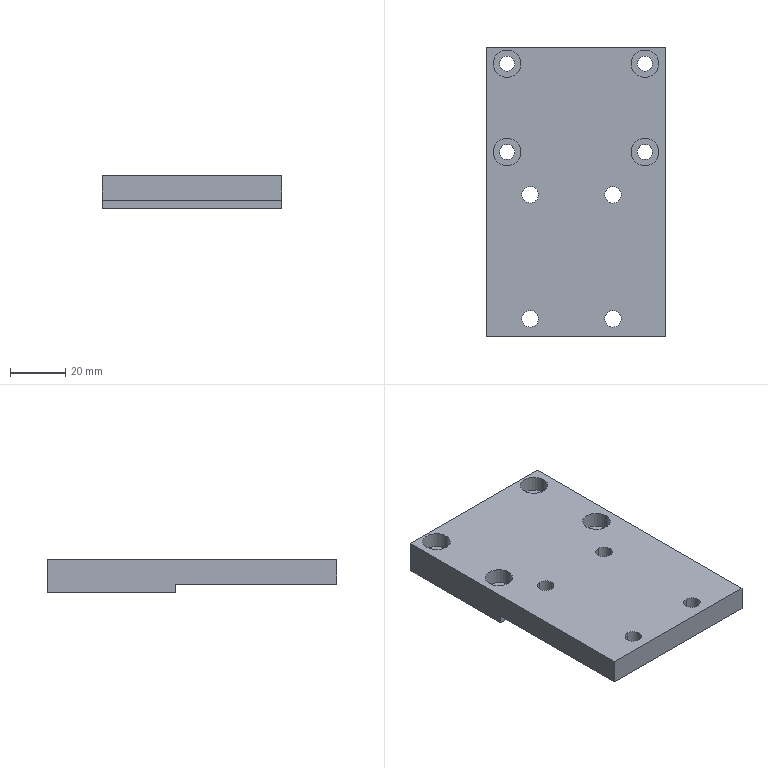Part | STEP file | X77B-02004 | 1 solid | 36 faces | box 65.2 x 105 x 12 mm | volume 67302 mm3 | cylinder 24 | plane 12 | commonest cylinder face diameters 5.5 x8 6 x8 10 x8
STEP:
#1=CARTESIAN_POINT('',(2707.241,69.988,12.));
#2=VERTEX_POINT('',#1);
#3=CARTESIAN_POINT('',(2707.241,75.988,12.));
#4=VERTEX_POINT('',#3);
#5=CARTESIAN_POINT('',(2707.241,72.988,12.));
#6=DIRECTION('',(0.,0.,-1.));
#7=DIRECTION('',(0.,1.,0.));
#8=AXIS2_PLACEMENT_3D('',#5,#6,#7);
#9=CIRCLE('',#8,3.);
#10=EDGE_CURVE('',#2,#4,#9,.T.);
#11=ORIENTED_EDGE('',*,*,#10,.F.);
#12=CARTESIAN_POINT('',(2707.241,69.988,3.));
#13=VERTEX_POINT('',#12);
#14=CARTESIAN_POINT('',(2707.241,69.988,3.));
#15=DIRECTION('',(0.,0.,-1.));
#16=VECTOR('',#15,1000.);
#17=LINE('',#14,#16);
#18=EDGE_CURVE('',#2,#13,#17,.T.);
#19=ORIENTED_EDGE('',*,*,#18,.T.);
#20=CARTESIAN_POINT('',(2707.241,75.988,3.));
#21=VERTEX_POINT('',#20);
#22=CARTESIAN_POINT('',(2707.241,72.988,3.));
#23=DIRECTION('',(0.,0.,-1.));
#24=DIRECTION('',(0.,1.,0.));
#25=AXIS2_PLACEMENT_3D('',#22,#23,#24);
#26=CIRCLE('',#25,3.);
#27=EDGE_CURVE('',#13,#21,#26,.T.);
#28=ORIENTED_EDGE('',*,*,#27,.T.);
#29=CARTESIAN_POINT('',(2707.241,75.988,3.));
#30=DIRECTION('',(0.,0.,-1.));
#31=VECTOR('',#30,1000.);
#32=LINE('',#29,#31);
#33=EDGE_CURVE('',#4,#21,#32,.T.);
#34=ORIENTED_EDGE('',*,*,#33,.F.);
#35=EDGE_LOOP('',(#11,#19,#28,#34));
#36=FACE_OUTER_BOUND('',#35,.T.);
#37=CARTESIAN_POINT('',(2707.241,72.988,3.));
#38=DIRECTION('',(0.,0.,-1.));
#39=DIRECTION('',(0.,1.,0.));
#40=AXIS2_PLACEMENT_3D('',#37,#38,#39);
#41=CYLINDRICAL_SURFACE('',#40,3.);
#42=ADVANCED_FACE('',(#36),#41,.F.);
#43=CARTESIAN_POINT('',(2737.241,69.988,12.));
#44=VERTEX_POINT('',#43);
#45=CARTESIAN_POINT('',(2737.241,75.988,12.));
#46=VERTEX_POINT('',#45);
#47=CARTESIAN_POINT('',(2737.241,72.988,12.));
#48=DIRECTION('',(0.,0.,-1.));
#49=DIRECTION('',(0.,1.,0.));
#50=AXIS2_PLACEMENT_3D('',#47,#48,#49);
#51=CIRCLE('',#50,3.);
#52=EDGE_CURVE('',#44,#46,#51,.T.);
#53=ORIENTED_EDGE('',*,*,#52,.F.);
#54=CARTESIAN_POINT('',(2737.241,69.988,3.));
#55=VERTEX_POINT('',#54);
#56=CARTESIAN_POINT('',(2737.241,69.988,3.));
#57=DIRECTION('',(0.,0.,-1.));
#58=VECTOR('',#57,1000.);
#59=LINE('',#56,#58);
#60=EDGE_CURVE('',#44,#55,#59,.T.);
#61=ORIENTED_EDGE('',*,*,#60,.T.);
#62=CARTESIAN_POINT('',(2737.241,75.988,3.));
#63=VERTEX_POINT('',#62);
#64=CARTESIAN_POINT('',(2737.241,72.988,3.));
#65=DIRECTION('',(0.,0.,-1.));
#66=DIRECTION('',(0.,1.,0.));
#67=AXIS2_PLACEMENT_3D('',#64,#65,#66);
#68=CIRCLE('',#67,3.);
#69=EDGE_CURVE('',#55,#63,#68,.T.);
#70=ORIENTED_EDGE('',*,*,#69,.T.);
#71=CARTESIAN_POINT('',(2737.241,75.988,3.));
#72=DIRECTION('',(0.,0.,-1.));
#73=VECTOR('',#72,1000.);
#74=LINE('',#71,#73);
#75=EDGE_CURVE('',#46,#63,#74,.T.);
#76=ORIENTED_EDGE('',*,*,#75,.F.);
#77=EDGE_LOOP('',(#53,#61,#70,#76));
#78=FACE_OUTER_BOUND('',#77,.T.);
#79=CARTESIAN_POINT('',(2737.241,72.988,3.));
#80=DIRECTION('',(0.,0.,-1.));
#81=DIRECTION('',(0.,1.,0.));
#82=AXIS2_PLACEMENT_3D('',#79,#80,#81);
#83=CYLINDRICAL_SURFACE('',#82,3.);
#84=ADVANCED_FACE('',(#78),#83,.F.);
#85=CARTESIAN_POINT('',(2707.241,24.988,12.));
#86=VERTEX_POINT('',#85);
#87=CARTESIAN_POINT('',(2707.241,30.988,12.));
#88=VERTEX_POINT('',#87);
#89=CARTESIAN_POINT('',(2707.241,27.988,12.));
#90=DIRECTION('',(0.,0.,-1.));
#91=DIRECTION('',(0.,1.,0.));
#92=AXIS2_PLACEMENT_3D('',#89,#90,#91);
#93=CIRCLE('',#92,3.);
#94=EDGE_CURVE('',#86,#88,#93,.T.);
#95=ORIENTED_EDGE('',*,*,#94,.F.);
#96=CARTESIAN_POINT('',(2707.241,24.988,3.));
#97=VERTEX_POINT('',#96);
#98=CARTESIAN_POINT('',(2707.241,24.988,3.));
#99=DIRECTION('',(0.,0.,-1.));
#100=VECTOR('',#99,1000.);
#101=LINE('',#98,#100);
#102=EDGE_CURVE('',#86,#97,#101,.T.);
#103=ORIENTED_EDGE('',*,*,#102,.T.);
#104=CARTESIAN_POINT('',(2707.241,30.988,3.));
#105=VERTEX_POINT('',#104);
#106=CARTESIAN_POINT('',(2707.241,27.988,3.));
#107=DIRECTION('',(0.,0.,-1.));
#108=DIRECTION('',(0.,1.,0.));
#109=AXIS2_PLACEMENT_3D('',#106,#107,#108);
#110=CIRCLE('',#109,3.);
#111=EDGE_CURVE('',#97,#105,#110,.T.);
#112=ORIENTED_EDGE('',*,*,#111,.T.);
#113=CARTESIAN_POINT('',(2707.241,30.988,3.));
#114=DIRECTION('',(0.,0.,-1.));
#115=VECTOR('',#114,1000.);
#116=LINE('',#113,#115);
#117=EDGE_CURVE('',#88,#105,#116,.T.);
#118=ORIENTED_EDGE('',*,*,#117,.F.);
#119=EDGE_LOOP('',(#95,#103,#112,#118));
#120=FACE_OUTER_BOUND('',#119,.T.);
#121=CARTESIAN_POINT('',(2707.241,27.988,3.));
#122=DIRECTION('',(0.,0.,-1.));
#123=DIRECTION('',(0.,1.,0.));
#124=AXIS2_PLACEMENT_3D('',#121,#122,#123);
#125=CYLINDRICAL_SURFACE('',#124,3.);
#126=ADVANCED_FACE('',(#120),#125,.F.);
#127=CARTESIAN_POINT('',(2737.241,24.988,12.));
#128=VERTEX_POINT('',#127);
#129=CARTESIAN_POINT('',(2737.241,30.988,12.));
#130=VERTEX_POINT('',#129);
#131=CARTESIAN_POINT('',(2737.241,27.988,12.));
#132=DIRECTION('',(0.,0.,-1.));
#133=DIRECTION('',(0.,1.,0.));
#134=AXIS2_PLACEMENT_3D('',#131,#132,#133);
#135=CIRCLE('',#134,3.);
#136=EDGE_CURVE('',#128,#130,#135,.T.);
#137=ORIENTED_EDGE('',*,*,#136,.F.);
#138=CARTESIAN_POINT('',(2737.241,24.988,3.));
#139=VERTEX_POINT('',#138);
#140=CARTESIAN_POINT('',(2737.241,24.988,3.));
#141=DIRECTION('',(0.,0.,-1.));
#142=VECTOR('',#141,1000.);
#143=LINE('',#140,#142);
#144=EDGE_CURVE('',#128,#139,#143,.T.);
#145=ORIENTED_EDGE('',*,*,#144,.T.);
#146=CARTESIAN_POINT('',(2737.241,30.988,3.));
#147=VERTEX_POINT('',#146);
#148=CARTESIAN_POINT('',(2737.241,27.988,3.));
#149=DIRECTION('',(0.,0.,-1.));
#150=DIRECTION('',(0.,1.,0.));
#151=AXIS2_PLACEMENT_3D('',#148,#149,#150);
#152=CIRCLE('',#151,3.);
#153=EDGE_CURVE('',#139,#147,#152,.T.);
#154=ORIENTED_EDGE('',*,*,#153,.T.);
#155=CARTESIAN_POINT('',(2737.241,30.988,3.));
#156=DIRECTION('',(0.,0.,-1.));
#157=VECTOR('',#156,1000.);
#158=LINE('',#155,#157);
#159=EDGE_CURVE('',#130,#147,#158,.T.);
#160=ORIENTED_EDGE('',*,*,#159,.F.);
#161=EDGE_LOOP('',(#137,#145,#154,#160));
#162=FACE_OUTER_BOUND('',#161,.T.);
#163=CARTESIAN_POINT('',(2737.241,27.988,3.));
#164=DIRECTION('',(0.,0.,-1.));
#165=DIRECTION('',(0.,1.,0.));
#166=AXIS2_PLACEMENT_3D('',#163,#164,#165);
#167=CYLINDRICAL_SURFACE('',#166,3.);
#168=ADVANCED_FACE('',(#162),#167,.F.);
#169=CARTESIAN_POINT('',(2693.841,120.488,6.3));
#170=VERTEX_POINT('',#169);
#171=CARTESIAN_POINT('',(2703.841,120.488,6.3));
#172=VERTEX_POINT('',#171);
#173=CARTESIAN_POINT('',(2698.841,120.488,6.3));
#174=DIRECTION('',(0.,0.,1.));
#175=DIRECTION('',(1.,0.,0.));
#176=AXIS2_PLACEMENT_3D('',#173,#174,#175);
#177=CIRCLE('',#176,5.);
#178=EDGE_CURVE('',#170,#172,#177,.T.);
#179=ORIENTED_EDGE('',*,*,#178,.F.);
#180=CARTESIAN_POINT('',(2693.841,120.488,12.));
#181=VERTEX_POINT('',#180);
#182=CARTESIAN_POINT('',(2693.841,120.488,12.));
#183=DIRECTION('',(0.,0.,1.));
#184=VECTOR('',#183,1000.);
#185=LINE('',#182,#184);
#186=EDGE_CURVE('',#170,#181,#185,.T.);
#187=ORIENTED_EDGE('',*,*,#186,.T.);
#188=CARTESIAN_POINT('',(2703.841,120.488,12.));
#189=VERTEX_POINT('',#188);
#190=CARTESIAN_POINT('',(2698.841,120.488,12.));
#191=DIRECTION('',(0.,0.,1.));
#192=DIRECTION('',(1.,0.,0.));
#193=AXIS2_PLACEMENT_3D('',#190,#191,#192);
#194=CIRCLE('',#193,5.);
#195=EDGE_CURVE('',#181,#189,#194,.T.);
#196=ORIENTED_EDGE('',*,*,#195,.T.);
#197=CARTESIAN_POINT('',(2703.841,120.488,12.));
#198=DIRECTION('',(0.,0.,1.));
#199=VECTOR('',#198,1000.);
#200=LINE('',#197,#199);
#201=EDGE_CURVE('',#172,#189,#200,.T.);
#202=ORIENTED_EDGE('',*,*,#201,.F.);
#203=EDGE_LOOP('',(#179,#187,#196,#202));
#204=FACE_OUTER_BOUND('',#203,.T.);
#205=CARTESIAN_POINT('',(2698.841,120.488,12.));
#206=DIRECTION('',(0.,0.,1.));
#207=DIRECTION('',(1.,0.,0.));
#208=AXIS2_PLACEMENT_3D('',#205,#206,#207);
#209=CYLINDRICAL_SURFACE('',#208,5.);
#210=ADVANCED_FACE('',(#204),#209,.F.);
#211=CARTESIAN_POINT('',(2696.091,120.488,0.));
#212=VERTEX_POINT('',#211);
#213=CARTESIAN_POINT('',(2701.591,120.488,0.));
#214=VERTEX_POINT('',#213);
#215=CARTESIAN_POINT('',(2698.841,120.488,0.));
#216=DIRECTION('',(0.,0.,1.));
#217=DIRECTION('',(1.,0.,0.));
#218=AXIS2_PLACEMENT_3D('',#215,#216,#217);
#219=CIRCLE('',#218,2.75);
#220=EDGE_CURVE('',#212,#214,#219,.T.);
#221=ORIENTED_EDGE('',*,*,#220,.F.);
#222=CARTESIAN_POINT('',(2696.091,120.488,6.3));
#223=VERTEX_POINT('',#222);
#224=CARTESIAN_POINT('',(2696.091,120.488,12.));
#225=DIRECTION('',(0.,0.,1.));
#226=VECTOR('',#225,1000.);
#227=LINE('',#224,#226);
#228=EDGE_CURVE('',#212,#223,#227,.T.);
#229=ORIENTED_EDGE('',*,*,#228,.T.);
#230=CARTESIAN_POINT('',(2701.591,120.488,6.3));
#231=VERTEX_POINT('',#230);
#232=CARTESIAN_POINT('',(2698.841,120.488,6.3));
#233=DIRECTION('',(0.,0.,1.));
#234=DIRECTION('',(1.,0.,0.));
#235=AXIS2_PLACEMENT_3D('',#232,#233,#234);
#236=CIRCLE('',#235,2.75);
#237=EDGE_CURVE('',#223,#231,#236,.T.);
#238=ORIENTED_EDGE('',*,*,#237,.T.);
#239=CARTESIAN_POINT('',(2701.591,120.488,12.));
#240=DIRECTION('',(0.,0.,1.));
#241=VECTOR('',#240,1000.);
#242=LINE('',#239,#241);
#243=EDGE_CURVE('',#214,#231,#242,.T.);
#244=ORIENTED_EDGE('',*,*,#243,.F.);
#245=EDGE_LOOP('',(#221,#229,#238,#244));
#246=FACE_OUTER_BOUND('',#245,.T.);
#247=CARTESIAN_POINT('',(2698.841,120.488,12.));
#248=DIRECTION('',(0.,0.,1.));
#249=DIRECTION('',(1.,0.,0.));
#250=AXIS2_PLACEMENT_3D('',#247,#248,#249);
#251=CYLINDRICAL_SURFACE('',#250,2.75);
#252=ADVANCED_FACE('',(#246),#251,.F.);
#253=CARTESIAN_POINT('',(2743.841,120.488,6.3));
#254=VERTEX_POINT('',#253);
#255=CARTESIAN_POINT('',(2753.841,120.488,6.3));
#256=VERTEX_POINT('',#255);
#257=CARTESIAN_POINT('',(2748.841,120.488,6.3));
#258=DIRECTION('',(0.,0.,1.));
#259=DIRECTION('',(1.,0.,0.));
#260=AXIS2_PLACEMENT_3D('',#257,#258,#259);
#261=CIRCLE('',#260,5.);
#262=EDGE_CURVE('',#254,#256,#261,.T.);
#263=ORIENTED_EDGE('',*,*,#262,.F.);
#264=CARTESIAN_POINT('',(2743.841,120.488,12.));
#265=VERTEX_POINT('',#264);
#266=CARTESIAN_POINT('',(2743.841,120.488,12.));
#267=DIRECTION('',(0.,0.,1.));
#268=VECTOR('',#267,1000.);
#269=LINE('',#266,#268);
#270=EDGE_CURVE('',#254,#265,#269,.T.);
#271=ORIENTED_EDGE('',*,*,#270,.T.);
#272=CARTESIAN_POINT('',(2753.841,120.488,12.));
#273=VERTEX_POINT('',#272);
#274=CARTESIAN_POINT('',(2748.841,120.488,12.));
#275=DIRECTION('',(0.,0.,1.));
#276=DIRECTION('',(1.,0.,0.));
#277=AXIS2_PLACEMENT_3D('',#274,#275,#276);
#278=CIRCLE('',#277,5.);
#279=EDGE_CURVE('',#265,#273,#278,.T.);
#280=ORIENTED_EDGE('',*,*,#279,.T.);
#281=CARTESIAN_POINT('',(2753.841,120.488,12.));
#282=DIRECTION('',(0.,0.,1.));
#283=VECTOR('',#282,1000.);
#284=LINE('',#281,#283);
#285=EDGE_CURVE('',#256,#273,#284,.T.);
#286=ORIENTED_EDGE('',*,*,#285,.F.);
#287=EDGE_LOOP('',(#263,#271,#280,#286));
#288=FACE_OUTER_BOUND('',#287,.T.);
#289=CARTESIAN_POINT('',(2748.841,120.488,12.));
#290=DIRECTION('',(0.,0.,1.));
#291=DIRECTION('',(1.,0.,0.));
#292=AXIS2_PLACEMENT_3D('',#289,#290,#291);
#293=CYLINDRICAL_SURFACE('',#292,5.);
#294=ADVANCED_FACE('',(#288),#293,.F.);
#295=CARTESIAN_POINT('',(2746.091,120.488,0.));
#296=VERTEX_POINT('',#295);
#297=CARTESIAN_POINT('',(2751.591,120.488,0.));
#298=VERTEX_POINT('',#297);
#299=CARTESIAN_POINT('',(2748.841,120.488,0.));
#300=DIRECTION('',(0.,0.,1.));
#301=DIRECTION('',(1.,0.,0.));
#302=AXIS2_PLACEMENT_3D('',#299,#300,#301);
#303=CIRCLE('',#302,2.75);
#304=EDGE_CURVE('',#296,#298,#303,.T.);
#305=ORIENTED_EDGE('',*,*,#304,.F.);
#306=CARTESIAN_POINT('',(2746.091,120.488,6.3));
#307=VERTEX_POINT('',#306);
#308=CARTESIAN_POINT('',(2746.091,120.488,12.));
#309=DIRECTION('',(0.,0.,1.));
#310=VECTOR('',#309,1000.);
#311=LINE('',#308,#310);
#312=EDGE_CURVE('',#296,#307,#311,.T.);
#313=ORIENTED_EDGE('',*,*,#312,.T.);
#314=CARTESIAN_POINT('',(2751.591,120.488,6.3));
#315=VERTEX_POINT('',#314);
#316=CARTESIAN_POINT('',(2748.841,120.488,6.3));
#317=DIRECTION('',(0.,0.,1.));
#318=DIRECTION('',(1.,0.,0.));
#319=AXIS2_PLACEMENT_3D('',#316,#317,#318);
#320=CIRCLE('',#319,2.75);
#321=EDGE_CURVE('',#307,#315,#320,.T.);
#322=ORIENTED_EDGE('',*,*,#321,.T.);
#323=CARTESIAN_POINT('',(2751.591,120.488,12.));
#324=DIRECTION('',(0.,0.,1.));
#325=VECTOR('',#324,1000.);
#326=LINE('',#323,#325);
#327=EDGE_CURVE('',#298,#315,#326,.T.);
#328=ORIENTED_EDGE('',*,*,#327,.F.);
#329=EDGE_LOOP('',(#305,#313,#322,#328));
#330=FACE_OUTER_BOUND('',#329,.T.);
#331=CARTESIAN_POINT('',(2748.841,120.488,12.));
#332=DIRECTION('',(0.,0.,1.));
#333=DIRECTION('',(1.,0.,0.));
#334=AXIS2_PLACEMENT_3D('',#331,#332,#333);
#335=CYLINDRICAL_SURFACE('',#334,2.75);
#336=ADVANCED_FACE('',(#330),#335,.F.);
#337=CARTESIAN_POINT('',(2743.841,88.488,6.3));
#338=VERTEX_POINT('',#337);
#339=CARTESIAN_POINT('',(2753.841,88.488,6.3));
#340=VERTEX_POINT('',#339);
#341=CARTESIAN_POINT('',(2748.841,88.488,6.3));
#342=DIRECTION('',(0.,0.,1.));
#343=DIRECTION('',(1.,0.,0.));
#344=AXIS2_PLACEMENT_3D('',#341,#342,#343);
#345=CIRCLE('',#344,5.);
#346=EDGE_CURVE('',#338,#340,#345,.T.);
#347=ORIENTED_EDGE('',*,*,#346,.F.);
#348=CARTESIAN_POINT('',(2743.841,88.488,12.));
#349=VERTEX_POINT('',#348);
#350=CARTESIAN_POINT('',(2743.841,88.488,12.));
#351=DIRECTION('',(0.,0.,1.));
#352=VECTOR('',#351,1000.);
#353=LINE('',#350,#352);
#354=EDGE_CURVE('',#338,#349,#353,.T.);
#355=ORIENTED_EDGE('',*,*,#354,.T.);
#356=CARTESIAN_POINT('',(2753.841,88.488,12.));
#357=VERTEX_POINT('',#356);
#358=CARTESIAN_POINT('',(2748.841,88.488,12.));
#359=DIRECTION('',(0.,0.,1.));
#360=DIRECTION('',(1.,0.,0.));
#361=AXIS2_PLACEMENT_3D('',#358,#359,#360);
#362=CIRCLE('',#361,5.);
#363=EDGE_CURVE('',#349,#357,#362,.T.);
#364=ORIENTED_EDGE('',*,*,#363,.T.);
#365=CARTESIAN_POINT('',(2753.841,88.488,12.));
#366=DIRECTION('',(0.,0.,1.));
#367=VECTOR('',#366,1000.);
#368=LINE('',#365,#367);
#369=EDGE_CURVE('',#340,#357,#368,.T.);
#370=ORIENTED_EDGE('',*,*,#369,.F.);
#371=EDGE_LOOP('',(#347,#355,#364,#370));
#372=FACE_OUTER_BOUND('',#371,.T.);
#373=CARTESIAN_POINT('',(2748.841,88.488,12.));
#374=DIRECTION('',(0.,0.,1.));
#375=DIRECTION('',(1.,0.,0.));
#376=AXIS2_PLACEMENT_3D('',#373,#374,#375);
#377=CYLINDRICAL_SURFACE('',#376,5.);
#378=ADVANCED_FACE('',(#372),#377,.F.);
#379=CARTESIAN_POINT('',(2746.091,88.488,0.));
#380=VERTEX_POINT('',#379);
#381=CARTESIAN_POINT('',(2751.591,88.488,0.));
#382=VERTEX_POINT('',#381);
#383=CARTESIAN_POINT('',(2748.841,88.488,0.));
#384=DIRECTION('',(0.,0.,1.));
#385=DIRECTION('',(1.,0.,0.));
#386=AXIS2_PLACEMENT_3D('',#383,#384,#385);
#387=CIRCLE('',#386,2.75);
#388=EDGE_CURVE('',#380,#382,#387,.T.);
#389=ORIENTED_EDGE('',*,*,#388,.F.);
#390=CARTESIAN_POINT('',(2746.091,88.488,6.3));
#391=VERTEX_POINT('',#390);
#392=CARTESIAN_POINT('',(2746.091,88.488,12.));
#393=DIRECTION('',(0.,0.,1.));
#394=VECTOR('',#393,1000.);
#395=LINE('',#392,#394);
#396=EDGE_CURVE('',#380,#391,#395,.T.);
#397=ORIENTED_EDGE('',*,*,#396,.T.);
#398=CARTESIAN_POINT('',(2751.591,88.488,6.3));
#399=VERTEX_POINT('',#398);
#400=CARTESIAN_POINT('',(2748.841,88.488,6.3));
#401=DIRECTION('',(0.,0.,1.));
#402=DIRECTION('',(1.,0.,0.));
#403=AXIS2_PLACEMENT_3D('',#400,#401,#402);
#404=CIRCLE('',#403,2.75);
#405=EDGE_CURVE('',#391,#399,#404,.T.);
#406=ORIENTED_EDGE('',*,*,#405,.T.);
#407=CARTESIAN_POINT('',(2751.591,88.488,12.));
#408=DIRECTION('',(0.,0.,1.));
#409=VECTOR('',#408,1000.);
#410=LINE('',#407,#409);
#411=EDGE_CURVE('',#382,#399,#410,.T.);
#412=ORIENTED_EDGE('',*,*,#411,.F.);
#413=EDGE_LOOP('',(#389,#397,#406,#412));
#414=FACE_OUTER_BOUND('',#413,.T.);
#415=CARTESIAN_POINT('',(2748.841,88.488,12.));
#416=DIRECTION('',(0.,0.,1.));
#417=DIRECTION('',(1.,0.,0.));
#418=AXIS2_PLACEMENT_3D('',#415,#416,#417);
#419=CYLINDRICAL_SURFACE('',#418,2.75);
#420=ADVANCED_FACE('',(#414),#419,.F.);
#421=CARTESIAN_POINT('',(2693.841,88.488,6.3));
#422=VERTEX_POINT('',#421);
#423=CARTESIAN_POINT('',(2703.841,88.488,6.3));
#424=VERTEX_POINT('',#423);
#425=CARTESIAN_POINT('',(2698.841,88.488,6.3));
#426=DIRECTION('',(0.,0.,1.));
#427=DIRECTION('',(1.,0.,0.));
#428=AXIS2_PLACEMENT_3D('',#425,#426,#427);
#429=CIRCLE('',#428,5.);
#430=EDGE_CURVE('',#422,#424,#429,.T.);
#431=ORIENTED_EDGE('',*,*,#430,.F.);
#432=CARTESIAN_POINT('',(2693.841,88.488,12.));
#433=VERTEX_POINT('',#432);
#434=CARTESIAN_POINT('',(2693.841,88.488,12.));
#435=DIRECTION('',(0.,0.,1.));
#436=VECTOR('',#435,1000.);
#437=LINE('',#434,#436);
#438=EDGE_CURVE('',#422,#433,#437,.T.);
#439=ORIENTED_EDGE('',*,*,#438,.T.);
#440=CARTESIAN_POINT('',(2703.841,88.488,12.));
#441=VERTEX_POINT('',#440);
#442=CARTESIAN_POINT('',(2698.841,88.488,12.));
#443=DIRECTION('',(0.,0.,1.));
#444=DIRECTION('',(1.,0.,0.));
#445=AXIS2_PLACEMENT_3D('',#442,#443,#444);
#446=CIRCLE('',#445,5.);
#447=EDGE_CURVE('',#433,#441,#446,.T.);
#448=ORIENTED_EDGE('',*,*,#447,.T.);
#449=CARTESIAN_POINT('',(2703.841,88.488,12.));
#450=DIRECTION('',(0.,0.,1.));
#451=VECTOR('',#450,1000.);
#452=LINE('',#449,#451);
#453=EDGE_CURVE('',#424,#441,#452,.T.);
#454=ORIENTED_EDGE('',*,*,#453,.F.);
#455=EDGE_LOOP('',(#431,#439,#448,#454));
#456=FACE_OUTER_BOUND('',#455,.T.);
#457=CARTESIAN_POINT('',(2698.841,88.488,12.));
#458=DIRECTION('',(0.,0.,1.));
#459=DIRECTION('',(1.,0.,0.));
#460=AXIS2_PLACEMENT_3D('',#457,#458,#459);
#461=CYLINDRICAL_SURFACE('',#460,5.);
#462=ADVANCED_FACE('',(#456),#461,.F.);
#463=CARTESIAN_POINT('',(2696.091,88.488,0.));
#464=VERTEX_POINT('',#463);
#465=CARTESIAN_POINT('',(2701.591,88.488,0.));
#466=VERTEX_POINT('',#465);
#467=CARTESIAN_POINT('',(2698.841,88.488,0.));
#468=DIRECTION('',(0.,0.,1.));
#469=DIRECTION('',(1.,0.,0.));
#470=AXIS2_PLACEMENT_3D('',#467,#468,#469);
#471=CIRCLE('',#470,2.75);
#472=EDGE_CURVE('',#464,#466,#471,.T.);
#473=ORIENTED_EDGE('',*,*,#472,.F.);
#474=CARTESIAN_POINT('',(2696.091,88.488,6.3));
#475=VERTEX_POINT('',#474);
#476=CARTESIAN_POINT('',(2696.091,88.488,12.));
#477=DIRECTION('',(0.,0.,1.));
#478=VECTOR('',#477,1000.);
#479=LINE('',#476,#478);
#480=EDGE_CURVE('',#464,#475,#479,.T.);
#481=ORIENTED_EDGE('',*,*,#480,.T.);
#482=CARTESIAN_POINT('',(2701.591,88.488,6.3));
#483=VERTEX_POINT('',#482);
#484=CARTESIAN_POINT('',(2698.841,88.488,6.3));
#485=DIRECTION('',(0.,0.,1.));
#486=DIRECTION('',(1.,0.,0.));
#487=AXIS2_PLACEMENT_3D('',#484,#485,#486);
#488=CIRCLE('',#487,2.75);
#489=EDGE_CURVE('',#475,#483,#488,.T.);
#490=ORIENTED_EDGE('',*,*,#489,.T.);
#491=CARTESIAN_POINT('',(2701.591,88.488,12.));
#492=DIRECTION('',(0.,0.,1.));
#493=VECTOR('',#492,1000.);
#494=LINE('',#491,#493);
#495=EDGE_CURVE('',#466,#483,#494,.T.);
#496=ORIENTED_EDGE('',*,*,#495,.F.);
#497=EDGE_LOOP('',(#473,#481,#490,#496));
#498=FACE_OUTER_BOUND('',#497,.T.);
#499=CARTESIAN_POINT('',(2698.841,88.488,12.));
#500=DIRECTION('',(0.,0.,1.));
#501=DIRECTION('',(1.,0.,0.));
#502=AXIS2_PLACEMENT_3D('',#499,#500,#501);
#503=CYLINDRICAL_SURFACE('',#502,2.75);
#504=ADVANCED_FACE('',(#498),#503,.F.);
#505=CARTESIAN_POINT('',(2691.241,79.988,0.));
#506=VERTEX_POINT('',#505);
#507=CARTESIAN_POINT('',(2691.241,79.988,3.));
#508=VERTEX_POINT('',#507);
#509=CARTESIAN_POINT('',(2691.241,79.988,0.));
#510=DIRECTION('',(0.,0.,1.));
#511=VECTOR('',#510,1000.);
#512=LINE('',#509,#511);
#513=EDGE_CURVE('',#506,#508,#512,.T.);
#514=ORIENTED_EDGE('',*,*,#513,.T.);
#515=CARTESIAN_POINT('',(2691.241,21.488,3.));
#516=VERTEX_POINT('',#515);
#517=CARTESIAN_POINT('',(2691.241,21.488,3.));
#518=DIRECTION('',(0.,-1.,0.));
#519=VECTOR('',#518,1000.);
#520=LINE('',#517,#519);
#521=EDGE_CURVE('',#508,#516,#520,.T.);
#522=ORIENTED_EDGE('',*,*,#521,.T.);
#523=CARTESIAN_POINT('',(2691.241,21.488,12.));
#524=VERTEX_POINT('',#523);
#525=CARTESIAN_POINT('',(2691.241,21.488,12.));
#526=DIRECTION('',(0.,0.,-1.));
#527=VECTOR('',#526,1000.);
#528=LINE('',#525,#527);
#529=EDGE_CURVE('',#524,#516,#528,.T.);
#530=ORIENTED_EDGE('',*,*,#529,.F.);
#531=CARTESIAN_POINT('',(2691.241,126.488,12.));
#532=VERTEX_POINT('',#531);
#533=CARTESIAN_POINT('',(2691.241,126.488,12.));
#534=DIRECTION('',(0.,-1.,0.));
#535=VECTOR('',#534,1000.);
#536=LINE('',#533,#535);
#537=EDGE_CURVE('',#532,#524,#536,.T.);
#538=ORIENTED_EDGE('',*,*,#537,.F.);
#539=CARTESIAN_POINT('',(2691.241,126.488,0.));
#540=VERTEX_POINT('',#539);
#541=CARTESIAN_POINT('',(2691.241,126.488,12.));
#542=DIRECTION('',(0.,0.,-1.));
#543=VECTOR('',#542,1000.);
#544=LINE('',#541,#543);
#545=EDGE_CURVE('',#532,#540,#544,.T.);
#546=ORIENTED_EDGE('',*,*,#545,.T.);
#547=CARTESIAN_POINT('',(2691.241,126.488,0.));
#548=DIRECTION('',(0.,-1.,0.));
#549=VECTOR('',#548,1000.);
#550=LINE('',#547,#549);
#551=EDGE_CURVE('',#540,#506,#550,.T.);
#552=ORIENTED_EDGE('',*,*,#551,.T.);
#553=EDGE_LOOP('',(#514,#522,#530,#538,#546,#552));
#554=FACE_OUTER_BOUND('',#553,.T.);
#555=CARTESIAN_POINT('',(2691.241,126.488,12.));
#556=DIRECTION('',(1.,0.,0.));
#557=DIRECTION('',(0.,0.,-1.));
#558=AXIS2_PLACEMENT_3D('',#555,#556,#557);
#559=PLANE('',#558);
#560=ADVANCED_FACE('',(#554),#559,.F.);
#561=ORIENTED_EDGE('',*,*,#529,.T.);
#562=CARTESIAN_POINT('',(2756.441,21.488,3.));
#563=VERTEX_POINT('',#562);
#564=CARTESIAN_POINT('',(2691.241,21.488,3.));
#565=DIRECTION('',(1.,0.,0.));
#566=VECTOR('',#565,1000.);
#567=LINE('',#564,#566);
#568=EDGE_CURVE('',#516,#563,#567,.T.);
#569=ORIENTED_EDGE('',*,*,#568,.T.);
#570=CARTESIAN_POINT('',(2756.441,21.488,12.));
#571=VERTEX_POINT('',#570);
#572=CARTESIAN_POINT('',(2756.441,21.488,12.));
#573=DIRECTION('',(0.,0.,-1.));
#574=VECTOR('',#573,1000.);
#575=LINE('',#572,#574);
#576=EDGE_CURVE('',#571,#563,#575,.T.);
#577=ORIENTED_EDGE('',*,*,#576,.F.);
#578=CARTESIAN_POINT('',(2691.241,21.488,12.));
#579=DIRECTION('',(1.,0.,0.));
#580=VECTOR('',#579,1000.);
#581=LINE('',#578,#580);
#582=EDGE_CURVE('',#524,#571,#581,.T.);
#583=ORIENTED_EDGE('',*,*,#582,.F.);
#584=EDGE_LOOP('',(#561,#569,#577,#583));
#585=FACE_OUTER_BOUND('',#584,.T.);
#586=CARTESIAN_POINT('',(2691.241,21.488,12.));
#587=DIRECTION('',(0.,1.,0.));
#588=DIRECTION('',(0.,0.,1.));
#589=AXIS2_PLACEMENT_3D('',#586,#587,#588);
#590=PLANE('',#589);
#591=ADVANCED_FACE('',(#585),#590,.F.);
#592=ORIENTED_EDGE('',*,*,#576,.T.);
#593=CARTESIAN_POINT('',(2756.441,79.988,3.));
#594=VERTEX_POINT('',#593);
#595=CARTESIAN_POINT('',(2756.441,21.488,3.));
#596=DIRECTION('',(0.,-1.,0.));
#597=VECTOR('',#596,1000.);
#598=LINE('',#595,#597);
#599=EDGE_CURVE('',#594,#563,#598,.T.);
#600=ORIENTED_EDGE('',*,*,#599,.F.);
#601=CARTESIAN_POINT('',(2756.441,79.988,0.));
#602=VERTEX_POINT('',#601);
#603=CARTESIAN_POINT('',(2756.441,79.988,0.));
#604=DIRECTION('',(0.,0.,1.));
#605=VECTOR('',#604,1000.);
#606=LINE('',#603,#605);
#607=EDGE_CURVE('',#602,#594,#606,.T.);
#608=ORIENTED_EDGE('',*,*,#607,.F.);
#609=CARTESIAN_POINT('',(2756.441,126.488,0.));
#610=VERTEX_POINT('',#609);
#611=CARTESIAN_POINT('',(2756.441,126.488,0.));
#612=DIRECTION('',(0.,1.,0.));
#613=VECTOR('',#612,1000.);
#614=LINE('',#611,#613);
#615=EDGE_CURVE('',#602,#610,#614,.T.);
#616=ORIENTED_EDGE('',*,*,#615,.T.);
#617=CARTESIAN_POINT('',(2756.441,126.488,12.));
#618=VERTEX_POINT('',#617);
#619=CARTESIAN_POINT('',(2756.441,126.488,12.));
#620=DIRECTION('',(0.,0.,-1.));
#621=VECTOR('',#620,1000.);
#622=LINE('',#619,#621);
#623=EDGE_CURVE('',#618,#610,#622,.T.);
#624=ORIENTED_EDGE('',*,*,#623,.F.);
#625=CARTESIAN_POINT('',(2756.441,126.488,12.));
#626=DIRECTION('',(0.,1.,0.));
#627=VECTOR('',#626,1000.);
#628=LINE('',#625,#627);
#629=EDGE_CURVE('',#571,#618,#628,.T.);
#630=ORIENTED_EDGE('',*,*,#629,.F.);
#631=EDGE_LOOP('',(#592,#600,#608,#616,#624,#630));
#632=FACE_OUTER_BOUND('',#631,.T.);
#633=CARTESIAN_POINT('',(2756.441,126.488,12.));
#634=DIRECTION('',(-1.,0.,0.));
#635=DIRECTION('',(0.,0.,1.));
#636=AXIS2_PLACEMENT_3D('',#633,#634,#635);
#637=PLANE('',#636);
#638=ADVANCED_FACE('',(#632),#637,.F.);
#639=CARTESIAN_POINT('',(2691.241,126.488,0.));
#640=DIRECTION('',(-1.,0.,0.));
#641=VECTOR('',#640,1000.);
#642=LINE('',#639,#641);
#643=EDGE_CURVE('',#610,#540,#642,.T.);
#644=ORIENTED_EDGE('',*,*,#643,.T.);
#645=ORIENTED_EDGE('',*,*,#545,.F.);
#646=CARTESIAN_POINT('',(2691.241,126.488,12.));
#647=DIRECTION('',(-1.,0.,0.));
#648=VECTOR('',#647,1000.);
#649=LINE('',#646,#648);
#650=EDGE_CURVE('',#618,#532,#649,.T.);
#651=ORIENTED_EDGE('',*,*,#650,.F.);
#652=ORIENTED_EDGE('',*,*,#623,.T.);
#653=EDGE_LOOP('',(#644,#645,#651,#652));
#654=FACE_OUTER_BOUND('',#653,.T.);
#655=CARTESIAN_POINT('',(2691.241,126.488,12.));
#656=DIRECTION('',(0.,-1.,0.));
#657=DIRECTION('',(0.,0.,-1.));
#658=AXIS2_PLACEMENT_3D('',#655,#656,#657);
#659=PLANE('',#658);
#660=ADVANCED_FACE('',(#654),#659,.F.);
#661=CARTESIAN_POINT('',(2707.241,72.988,12.));
#662=DIRECTION('',(0.,0.,-1.));
#663=DIRECTION('',(0.,1.,0.));
#664=AXIS2_PLACEMENT_3D('',#661,#662,#663);
#665=CIRCLE('',#664,3.);
#666=EDGE_CURVE('',#4,#2,#665,.T.);
#667=ORIENTED_EDGE('',*,*,#666,.T.);
#668=ORIENTED_EDGE('',*,*,#10,.T.);
#669=EDGE_LOOP('',(#667,#668));
#670=FACE_BOUND('',#669,.T.);
#671=CARTESIAN_POINT('',(2737.241,72.988,12.));
#672=DIRECTION('',(0.,0.,-1.));
#673=DIRECTION('',(0.,1.,0.));
#674=AXIS2_PLACEMENT_3D('',#671,#672,#673);
#675=CIRCLE('',#674,3.);
#676=EDGE_CURVE('',#46,#44,#675,.T.);
#677=ORIENTED_EDGE('',*,*,#676,.T.);
#678=ORIENTED_EDGE('',*,*,#52,.T.);
#679=EDGE_LOOP('',(#677,#678));
#680=FACE_BOUND('',#679,.T.);
#681=CARTESIAN_POINT('',(2707.241,27.988,12.));
#682=DIRECTION('',(0.,0.,-1.));
#683=DIRECTION('',(0.,1.,0.));
#684=AXIS2_PLACEMENT_3D('',#681,#682,#683);
#685=CIRCLE('',#684,3.);
#686=EDGE_CURVE('',#88,#86,#685,.T.);
#687=ORIENTED_EDGE('',*,*,#686,.T.);
#688=ORIENTED_EDGE('',*,*,#94,.T.);
#689=EDGE_LOOP('',(#687,#688));
#690=FACE_BOUND('',#689,.T.);
#691=CARTESIAN_POINT('',(2737.241,27.988,12.));
#692=DIRECTION('',(0.,0.,-1.));
#693=DIRECTION('',(0.,1.,0.));
#694=AXIS2_PLACEMENT_3D('',#691,#692,#693);
#695=CIRCLE('',#694,3.);
#696=EDGE_CURVE('',#130,#128,#695,.T.);
#697=ORIENTED_EDGE('',*,*,#696,.T.);
#698=ORIENTED_EDGE('',*,*,#136,.T.);
#699=EDGE_LOOP('',(#697,#698));
#700=FACE_BOUND('',#699,.T.);
#701=CARTESIAN_POINT('',(2698.841,120.488,12.));
#702=DIRECTION('',(0.,0.,1.));
#703=DIRECTION('',(1.,0.,0.));
#704=AXIS2_PLACEMENT_3D('',#701,#702,#703);
#705=CIRCLE('',#704,5.);
#706=EDGE_CURVE('',#189,#181,#705,.T.);
#707=ORIENTED_EDGE('',*,*,#706,.F.);
#708=ORIENTED_EDGE('',*,*,#195,.F.);
#709=EDGE_LOOP('',(#707,#708));
#710=FACE_BOUND('',#709,.T.);
#711=CARTESIAN_POINT('',(2748.841,120.488,12.));
#712=DIRECTION('',(0.,0.,1.));
#713=DIRECTION('',(1.,0.,0.));
#714=AXIS2_PLACEMENT_3D('',#711,#712,#713);
#715=CIRCLE('',#714,5.);
#716=EDGE_CURVE('',#273,#265,#715,.T.);
#717=ORIENTED_EDGE('',*,*,#716,.F.);
#718=ORIENTED_EDGE('',*,*,#279,.F.);
#719=EDGE_LOOP('',(#717,#718));
#720=FACE_BOUND('',#719,.T.);
#721=CARTESIAN_POINT('',(2748.841,88.488,12.));
#722=DIRECTION('',(0.,0.,1.));
#723=DIRECTION('',(1.,0.,0.));
#724=AXIS2_PLACEMENT_3D('',#721,#722,#723);
#725=CIRCLE('',#724,5.);
#726=EDGE_CURVE('',#357,#349,#725,.T.);
#727=ORIENTED_EDGE('',*,*,#726,.F.);
#728=ORIENTED_EDGE('',*,*,#363,.F.);
#729=EDGE_LOOP('',(#727,#728));
#730=FACE_BOUND('',#729,.T.);
#731=CARTESIAN_POINT('',(2698.841,88.488,12.));
#732=DIRECTION('',(0.,0.,1.));
#733=DIRECTION('',(1.,0.,0.));
#734=AXIS2_PLACEMENT_3D('',#731,#732,#733);
#735=CIRCLE('',#734,5.);
#736=EDGE_CURVE('',#441,#433,#735,.T.);
#737=ORIENTED_EDGE('',*,*,#736,.F.);
#738=ORIENTED_EDGE('',*,*,#447,.F.);
#739=EDGE_LOOP('',(#737,#738));
#740=FACE_BOUND('',#739,.T.);
#741=ORIENTED_EDGE('',*,*,#537,.T.);
#742=ORIENTED_EDGE('',*,*,#582,.T.);
#743=ORIENTED_EDGE('',*,*,#629,.T.);
#744=ORIENTED_EDGE('',*,*,#650,.T.);
#745=EDGE_LOOP('',(#741,#742,#743,#744));
#746=FACE_OUTER_BOUND('',#745,.T.);
#747=CARTESIAN_POINT('',(2691.241,21.488,12.));
#748=DIRECTION('',(0.,0.,1.));
#749=DIRECTION('',(1.,0.,0.));
#750=AXIS2_PLACEMENT_3D('',#747,#748,#749);
#751=PLANE('',#750);
#752=ADVANCED_FACE('',(#670,#680,#690,#700,#710,#720,#730,#740,#746),#751,.T.);
#753=CARTESIAN_POINT('',(2698.841,120.488,0.));
#754=DIRECTION('',(0.,0.,1.));
#755=DIRECTION('',(1.,0.,0.));
#756=AXIS2_PLACEMENT_3D('',#753,#754,#755);
#757=CIRCLE('',#756,2.75);
#758=EDGE_CURVE('',#214,#212,#757,.T.);
#759=ORIENTED_EDGE('',*,*,#758,.T.);
#760=ORIENTED_EDGE('',*,*,#220,.T.);
#761=EDGE_LOOP('',(#759,#760));
#762=FACE_BOUND('',#761,.T.);
#763=CARTESIAN_POINT('',(2748.841,120.488,0.));
#764=DIRECTION('',(0.,0.,1.));
#765=DIRECTION('',(1.,0.,0.));
#766=AXIS2_PLACEMENT_3D('',#763,#764,#765);
#767=CIRCLE('',#766,2.75);
#768=EDGE_CURVE('',#298,#296,#767,.T.);
#769=ORIENTED_EDGE('',*,*,#768,.T.);
#770=ORIENTED_EDGE('',*,*,#304,.T.);
#771=EDGE_LOOP('',(#769,#770));
#772=FACE_BOUND('',#771,.T.);
#773=CARTESIAN_POINT('',(2748.841,88.488,0.));
#774=DIRECTION('',(0.,0.,1.));
#775=DIRECTION('',(1.,0.,0.));
#776=AXIS2_PLACEMENT_3D('',#773,#774,#775);
#777=CIRCLE('',#776,2.75);
#778=EDGE_CURVE('',#382,#380,#777,.T.);
#779=ORIENTED_EDGE('',*,*,#778,.T.);
#780=ORIENTED_EDGE('',*,*,#388,.T.);
#781=EDGE_LOOP('',(#779,#780));
#782=FACE_BOUND('',#781,.T.);
#783=CARTESIAN_POINT('',(2698.841,88.488,0.));
#784=DIRECTION('',(0.,0.,1.));
#785=DIRECTION('',(1.,0.,0.));
#786=AXIS2_PLACEMENT_3D('',#783,#784,#785);
#787=CIRCLE('',#786,2.75);
#788=EDGE_CURVE('',#466,#464,#787,.T.);
#789=ORIENTED_EDGE('',*,*,#788,.T.);
#790=ORIENTED_EDGE('',*,*,#472,.T.);
#791=EDGE_LOOP('',(#789,#790));
#792=FACE_BOUND('',#791,.T.);
#793=ORIENTED_EDGE('',*,*,#615,.F.);
#794=CARTESIAN_POINT('',(2691.241,79.988,0.));
#795=DIRECTION('',(1.,0.,0.));
#796=VECTOR('',#795,1000.);
#797=LINE('',#794,#796);
#798=EDGE_CURVE('',#506,#602,#797,.T.);
#799=ORIENTED_EDGE('',*,*,#798,.F.);
#800=ORIENTED_EDGE('',*,*,#551,.F.);
#801=ORIENTED_EDGE('',*,*,#643,.F.);
#802=EDGE_LOOP('',(#793,#799,#800,#801));
#803=FACE_OUTER_BOUND('',#802,.T.);
#804=CARTESIAN_POINT('',(2691.241,21.488,0.));
#805=DIRECTION('',(0.,0.,1.));
#806=DIRECTION('',(1.,0.,0.));
#807=AXIS2_PLACEMENT_3D('',#804,#805,#806);
#808=PLANE('',#807);
#809=ADVANCED_FACE('',(#762,#772,#782,#792,#803),#808,.F.);
#810=CARTESIAN_POINT('',(2707.241,72.988,3.));
#811=DIRECTION('',(0.,0.,-1.));
#812=DIRECTION('',(0.,1.,0.));
#813=AXIS2_PLACEMENT_3D('',#810,#811,#812);
#814=CIRCLE('',#813,3.);
#815=EDGE_CURVE('',#21,#13,#814,.T.);
#816=ORIENTED_EDGE('',*,*,#815,.F.);
#817=ORIENTED_EDGE('',*,*,#27,.F.);
#818=EDGE_LOOP('',(#816,#817));
#819=FACE_BOUND('',#818,.T.);
#820=CARTESIAN_POINT('',(2737.241,72.988,3.));
#821=DIRECTION('',(0.,0.,-1.));
#822=DIRECTION('',(0.,1.,0.));
#823=AXIS2_PLACEMENT_3D('',#820,#821,#822);
#824=CIRCLE('',#823,3.);
#825=EDGE_CURVE('',#63,#55,#824,.T.);
#826=ORIENTED_EDGE('',*,*,#825,.F.);
#827=ORIENTED_EDGE('',*,*,#69,.F.);
#828=EDGE_LOOP('',(#826,#827));
#829=FACE_BOUND('',#828,.T.);
#830=CARTESIAN_POINT('',(2707.241,27.988,3.));
#831=DIRECTION('',(0.,0.,-1.));
#832=DIRECTION('',(0.,1.,0.));
#833=AXIS2_PLACEMENT_3D('',#830,#831,#832);
#834=CIRCLE('',#833,3.);
#835=EDGE_CURVE('',#105,#97,#834,.T.);
#836=ORIENTED_EDGE('',*,*,#835,.F.);
#837=ORIENTED_EDGE('',*,*,#111,.F.);
#838=EDGE_LOOP('',(#836,#837));
#839=FACE_BOUND('',#838,.T.);
#840=CARTESIAN_POINT('',(2737.241,27.988,3.));
#841=DIRECTION('',(0.,0.,-1.));
#842=DIRECTION('',(0.,1.,0.));
#843=AXIS2_PLACEMENT_3D('',#840,#841,#842);
#844=CIRCLE('',#843,3.);
#845=EDGE_CURVE('',#147,#139,#844,.T.);
#846=ORIENTED_EDGE('',*,*,#845,.F.);
#847=ORIENTED_EDGE('',*,*,#153,.F.);
#848=EDGE_LOOP('',(#846,#847));
#849=FACE_BOUND('',#848,.T.);
#850=ORIENTED_EDGE('',*,*,#599,.T.);
#851=ORIENTED_EDGE('',*,*,#568,.F.);
#852=ORIENTED_EDGE('',*,*,#521,.F.);
#853=CARTESIAN_POINT('',(2691.241,79.988,3.));
#854=DIRECTION('',(1.,0.,0.));
#855=VECTOR('',#854,1000.);
#856=LINE('',#853,#855);
#857=EDGE_CURVE('',#508,#594,#856,.T.);
#858=ORIENTED_EDGE('',*,*,#857,.T.);
#859=EDGE_LOOP('',(#850,#851,#852,#858));
#860=FACE_OUTER_BOUND('',#859,.T.);
#861=CARTESIAN_POINT('',(2691.241,21.488,3.));
#862=DIRECTION('',(0.,0.,1.));
#863=DIRECTION('',(0.,-1.,0.));
#864=AXIS2_PLACEMENT_3D('',#861,#862,#863);
#865=PLANE('',#864);
#866=ADVANCED_FACE('',(#819,#829,#839,#849,#860),#865,.F.);
#867=ORIENTED_EDGE('',*,*,#607,.T.);
#868=ORIENTED_EDGE('',*,*,#857,.F.);
#869=ORIENTED_EDGE('',*,*,#513,.F.);
#870=ORIENTED_EDGE('',*,*,#798,.T.);
#871=EDGE_LOOP('',(#867,#868,#869,#870));
#872=FACE_OUTER_BOUND('',#871,.T.);
#873=CARTESIAN_POINT('',(2691.241,79.988,0.));
#874=DIRECTION('',(0.,1.,0.));
#875=DIRECTION('',(0.,0.,1.));
#876=AXIS2_PLACEMENT_3D('',#873,#874,#875);
#877=PLANE('',#876);
#878=ADVANCED_FACE('',(#872),#877,.F.);
#879=ORIENTED_EDGE('',*,*,#480,.F.);
#880=ORIENTED_EDGE('',*,*,#788,.F.);
#881=ORIENTED_EDGE('',*,*,#495,.T.);
#882=CARTESIAN_POINT('',(2698.841,88.488,6.3));
#883=DIRECTION('',(0.,0.,1.));
#884=DIRECTION('',(1.,0.,0.));
#885=AXIS2_PLACEMENT_3D('',#882,#883,#884);
#886=CIRCLE('',#885,2.75);
#887=EDGE_CURVE('',#483,#475,#886,.T.);
#888=ORIENTED_EDGE('',*,*,#887,.T.);
#889=EDGE_LOOP('',(#879,#880,#881,#888));
#890=FACE_OUTER_BOUND('',#889,.T.);
#891=CARTESIAN_POINT('',(2698.841,88.488,12.));
#892=DIRECTION('',(0.,0.,1.));
#893=DIRECTION('',(1.,0.,0.));
#894=AXIS2_PLACEMENT_3D('',#891,#892,#893);
#895=CYLINDRICAL_SURFACE('',#894,2.75);
#896=ADVANCED_FACE('',(#890),#895,.F.);
#897=ORIENTED_EDGE('',*,*,#887,.F.);
#898=ORIENTED_EDGE('',*,*,#489,.F.);
#899=EDGE_LOOP('',(#897,#898));
#900=FACE_BOUND('',#899,.T.);
#901=CARTESIAN_POINT('',(2698.841,88.488,6.3));
#902=DIRECTION('',(0.,0.,1.));
#903=DIRECTION('',(1.,0.,0.));
#904=AXIS2_PLACEMENT_3D('',#901,#902,#903);
#905=CIRCLE('',#904,5.);
#906=EDGE_CURVE('',#424,#422,#905,.T.);
#907=ORIENTED_EDGE('',*,*,#906,.T.);
#908=ORIENTED_EDGE('',*,*,#430,.T.);
#909=EDGE_LOOP('',(#907,#908));
#910=FACE_OUTER_BOUND('',#909,.T.);
#911=CARTESIAN_POINT('',(2701.591,88.488,6.3));
#912=DIRECTION('',(0.,0.,-1.));
#913=DIRECTION('',(-1.,0.,0.));
#914=AXIS2_PLACEMENT_3D('',#911,#912,#913);
#915=PLANE('',#914);
#916=ADVANCED_FACE('',(#900,#910),#915,.F.);
#917=ORIENTED_EDGE('',*,*,#438,.F.);
#918=ORIENTED_EDGE('',*,*,#906,.F.);
#919=ORIENTED_EDGE('',*,*,#453,.T.);
#920=ORIENTED_EDGE('',*,*,#736,.T.);
#921=EDGE_LOOP('',(#917,#918,#919,#920));
#922=FACE_OUTER_BOUND('',#921,.T.);
#923=CARTESIAN_POINT('',(2698.841,88.488,12.));
#924=DIRECTION('',(0.,0.,1.));
#925=DIRECTION('',(1.,0.,0.));
#926=AXIS2_PLACEMENT_3D('',#923,#924,#925);
#927=CYLINDRICAL_SURFACE('',#926,5.);
#928=ADVANCED_FACE('',(#922),#927,.F.);
#929=ORIENTED_EDGE('',*,*,#396,.F.);
#930=ORIENTED_EDGE('',*,*,#778,.F.);
#931=ORIENTED_EDGE('',*,*,#411,.T.);
#932=CARTESIAN_POINT('',(2748.841,88.488,6.3));
#933=DIRECTION('',(0.,0.,1.));
#934=DIRECTION('',(1.,0.,0.));
#935=AXIS2_PLACEMENT_3D('',#932,#933,#934);
#936=CIRCLE('',#935,2.75);
#937=EDGE_CURVE('',#399,#391,#936,.T.);
#938=ORIENTED_EDGE('',*,*,#937,.T.);
#939=EDGE_LOOP('',(#929,#930,#931,#938));
#940=FACE_OUTER_BOUND('',#939,.T.);
#941=CARTESIAN_POINT('',(2748.841,88.488,12.));
#942=DIRECTION('',(0.,0.,1.));
#943=DIRECTION('',(1.,0.,0.));
#944=AXIS2_PLACEMENT_3D('',#941,#942,#943);
#945=CYLINDRICAL_SURFACE('',#944,2.75);
#946=ADVANCED_FACE('',(#940),#945,.F.);
#947=ORIENTED_EDGE('',*,*,#937,.F.);
#948=ORIENTED_EDGE('',*,*,#405,.F.);
#949=EDGE_LOOP('',(#947,#948));
#950=FACE_BOUND('',#949,.T.);
#951=CARTESIAN_POINT('',(2748.841,88.488,6.3));
#952=DIRECTION('',(0.,0.,1.));
#953=DIRECTION('',(1.,0.,0.));
#954=AXIS2_PLACEMENT_3D('',#951,#952,#953);
#955=CIRCLE('',#954,5.);
#956=EDGE_CURVE('',#340,#338,#955,.T.);
#957=ORIENTED_EDGE('',*,*,#956,.T.);
#958=ORIENTED_EDGE('',*,*,#346,.T.);
#959=EDGE_LOOP('',(#957,#958));
#960=FACE_OUTER_BOUND('',#959,.T.);
#961=CARTESIAN_POINT('',(2751.591,88.488,6.3));
#962=DIRECTION('',(0.,0.,-1.));
#963=DIRECTION('',(-1.,0.,0.));
#964=AXIS2_PLACEMENT_3D('',#961,#962,#963);
#965=PLANE('',#964);
#966=ADVANCED_FACE('',(#950,#960),#965,.F.);
#967=ORIENTED_EDGE('',*,*,#354,.F.);
#968=ORIENTED_EDGE('',*,*,#956,.F.);
#969=ORIENTED_EDGE('',*,*,#369,.T.);
#970=ORIENTED_EDGE('',*,*,#726,.T.);
#971=EDGE_LOOP('',(#967,#968,#969,#970));
#972=FACE_OUTER_BOUND('',#971,.T.);
#973=CARTESIAN_POINT('',(2748.841,88.488,12.));
#974=DIRECTION('',(0.,0.,1.));
#975=DIRECTION('',(1.,0.,0.));
#976=AXIS2_PLACEMENT_3D('',#973,#974,#975);
#977=CYLINDRICAL_SURFACE('',#976,5.);
#978=ADVANCED_FACE('',(#972),#977,.F.);
#979=ORIENTED_EDGE('',*,*,#312,.F.);
#980=ORIENTED_EDGE('',*,*,#768,.F.);
#981=ORIENTED_EDGE('',*,*,#327,.T.);
#982=CARTESIAN_POINT('',(2748.841,120.488,6.3));
#983=DIRECTION('',(0.,0.,1.));
#984=DIRECTION('',(1.,0.,0.));
#985=AXIS2_PLACEMENT_3D('',#982,#983,#984);
#986=CIRCLE('',#985,2.75);
#987=EDGE_CURVE('',#315,#307,#986,.T.);
#988=ORIENTED_EDGE('',*,*,#987,.T.);
#989=EDGE_LOOP('',(#979,#980,#981,#988));
#990=FACE_OUTER_BOUND('',#989,.T.);
#991=CARTESIAN_POINT('',(2748.841,120.488,12.));
#992=DIRECTION('',(0.,0.,1.));
#993=DIRECTION('',(1.,0.,0.));
#994=AXIS2_PLACEMENT_3D('',#991,#992,#993);
#995=CYLINDRICAL_SURFACE('',#994,2.75);
#996=ADVANCED_FACE('',(#990),#995,.F.);
#997=ORIENTED_EDGE('',*,*,#987,.F.);
#998=ORIENTED_EDGE('',*,*,#321,.F.);
#999=EDGE_LOOP('',(#997,#998));
#1000=FACE_BOUND('',#999,.T.);
#1001=CARTESIAN_POINT('',(2748.841,120.488,6.3));
#1002=DIRECTION('',(0.,0.,1.));
#1003=DIRECTION('',(1.,0.,0.));
#1004=AXIS2_PLACEMENT_3D('',#1001,#1002,#1003);
#1005=CIRCLE('',#1004,5.);
#1006=EDGE_CURVE('',#256,#254,#1005,.T.);
#1007=ORIENTED_EDGE('',*,*,#1006,.T.);
#1008=ORIENTED_EDGE('',*,*,#262,.T.);
#1009=EDGE_LOOP('',(#1007,#1008));
#1010=FACE_OUTER_BOUND('',#1009,.T.);
#1011=CARTESIAN_POINT('',(2751.591,120.488,6.3));
#1012=DIRECTION('',(0.,0.,-1.));
#1013=DIRECTION('',(-1.,0.,0.));
#1014=AXIS2_PLACEMENT_3D('',#1011,#1012,#1013);
#1015=PLANE('',#1014);
#1016=ADVANCED_FACE('',(#1000,#1010),#1015,.F.);
#1017=ORIENTED_EDGE('',*,*,#270,.F.);
#1018=ORIENTED_EDGE('',*,*,#1006,.F.);
#1019=ORIENTED_EDGE('',*,*,#285,.T.);
#1020=ORIENTED_EDGE('',*,*,#716,.T.);
#1021=EDGE_LOOP('',(#1017,#1018,#1019,#1020));
#1022=FACE_OUTER_BOUND('',#1021,.T.);
#1023=CARTESIAN_POINT('',(2748.841,120.488,12.));
#1024=DIRECTION('',(0.,0.,1.));
#1025=DIRECTION('',(1.,0.,0.));
#1026=AXIS2_PLACEMENT_3D('',#1023,#1024,#1025);
#1027=CYLINDRICAL_SURFACE('',#1026,5.);
#1028=ADVANCED_FACE('',(#1022),#1027,.F.);
#1029=ORIENTED_EDGE('',*,*,#228,.F.);
#1030=ORIENTED_EDGE('',*,*,#758,.F.);
#1031=ORIENTED_EDGE('',*,*,#243,.T.);
#1032=CARTESIAN_POINT('',(2698.841,120.488,6.3));
#1033=DIRECTION('',(0.,0.,1.));
#1034=DIRECTION('',(1.,0.,0.));
#1035=AXIS2_PLACEMENT_3D('',#1032,#1033,#1034);
#1036=CIRCLE('',#1035,2.75);
#1037=EDGE_CURVE('',#231,#223,#1036,.T.);
#1038=ORIENTED_EDGE('',*,*,#1037,.T.);
#1039=EDGE_LOOP('',(#1029,#1030,#1031,#1038));
#1040=FACE_OUTER_BOUND('',#1039,.T.);
#1041=CARTESIAN_POINT('',(2698.841,120.488,12.));
#1042=DIRECTION('',(0.,0.,1.));
#1043=DIRECTION('',(1.,0.,0.));
#1044=AXIS2_PLACEMENT_3D('',#1041,#1042,#1043);
#1045=CYLINDRICAL_SURFACE('',#1044,2.75);
#1046=ADVANCED_FACE('',(#1040),#1045,.F.);
#1047=ORIENTED_EDGE('',*,*,#1037,.F.);
#1048=ORIENTED_EDGE('',*,*,#237,.F.);
#1049=EDGE_LOOP('',(#1047,#1048));
#1050=FACE_BOUND('',#1049,.T.);
#1051=CARTESIAN_POINT('',(2698.841,120.488,6.3));
#1052=DIRECTION('',(0.,0.,1.));
#1053=DIRECTION('',(1.,0.,0.));
#1054=AXIS2_PLACEMENT_3D('',#1051,#1052,#1053);
#1055=CIRCLE('',#1054,5.);
#1056=EDGE_CURVE('',#172,#170,#1055,.T.);
#1057=ORIENTED_EDGE('',*,*,#1056,.T.);
#1058=ORIENTED_EDGE('',*,*,#178,.T.);
#1059=EDGE_LOOP('',(#1057,#1058));
#1060=FACE_OUTER_BOUND('',#1059,.T.);
#1061=CARTESIAN_POINT('',(2701.591,120.488,6.3));
#1062=DIRECTION('',(0.,0.,-1.));
#1063=DIRECTION('',(-1.,0.,0.));
#1064=AXIS2_PLACEMENT_3D('',#1061,#1062,#1063);
#1065=PLANE('',#1064);
#1066=ADVANCED_FACE('',(#1050,#1060),#1065,.F.);
#1067=ORIENTED_EDGE('',*,*,#186,.F.);
#1068=ORIENTED_EDGE('',*,*,#1056,.F.);
#1069=ORIENTED_EDGE('',*,*,#201,.T.);
#1070=ORIENTED_EDGE('',*,*,#706,.T.);
#1071=EDGE_LOOP('',(#1067,#1068,#1069,#1070));
#1072=FACE_OUTER_BOUND('',#1071,.T.);
#1073=CARTESIAN_POINT('',(2698.841,120.488,12.));
#1074=DIRECTION('',(0.,0.,1.));
#1075=DIRECTION('',(1.,0.,0.));
#1076=AXIS2_PLACEMENT_3D('',#1073,#1074,#1075);
#1077=CYLINDRICAL_SURFACE('',#1076,5.);
#1078=ADVANCED_FACE('',(#1072),#1077,.F.);
#1079=ORIENTED_EDGE('',*,*,#144,.F.);
#1080=ORIENTED_EDGE('',*,*,#696,.F.);
#1081=ORIENTED_EDGE('',*,*,#159,.T.);
#1082=ORIENTED_EDGE('',*,*,#845,.T.);
#1083=EDGE_LOOP('',(#1079,#1080,#1081,#1082));
#1084=FACE_OUTER_BOUND('',#1083,.T.);
#1085=CARTESIAN_POINT('',(2737.241,27.988,3.));
#1086=DIRECTION('',(0.,0.,-1.));
#1087=DIRECTION('',(0.,1.,0.));
#1088=AXIS2_PLACEMENT_3D('',#1085,#1086,#1087);
#1089=CYLINDRICAL_SURFACE('',#1088,3.);
#1090=ADVANCED_FACE('',(#1084),#1089,.F.);
#1091=ORIENTED_EDGE('',*,*,#102,.F.);
#1092=ORIENTED_EDGE('',*,*,#686,.F.);
#1093=ORIENTED_EDGE('',*,*,#117,.T.);
#1094=ORIENTED_EDGE('',*,*,#835,.T.);
#1095=EDGE_LOOP('',(#1091,#1092,#1093,#1094));
#1096=FACE_OUTER_BOUND('',#1095,.T.);
#1097=CARTESIAN_POINT('',(2707.241,27.988,3.));
#1098=DIRECTION('',(0.,0.,-1.));
#1099=DIRECTION('',(0.,1.,0.));
#1100=AXIS2_PLACEMENT_3D('',#1097,#1098,#1099);
#1101=CYLINDRICAL_SURFACE('',#1100,3.);
#1102=ADVANCED_FACE('',(#1096),#1101,.F.);
#1103=ORIENTED_EDGE('',*,*,#60,.F.);
#1104=ORIENTED_EDGE('',*,*,#676,.F.);
#1105=ORIENTED_EDGE('',*,*,#75,.T.);
#1106=ORIENTED_EDGE('',*,*,#825,.T.);
#1107=EDGE_LOOP('',(#1103,#1104,#1105,#1106));
#1108=FACE_OUTER_BOUND('',#1107,.T.);
#1109=CARTESIAN_POINT('',(2737.241,72.988,3.));
#1110=DIRECTION('',(0.,0.,-1.));
#1111=DIRECTION('',(0.,1.,0.));
#1112=AXIS2_PLACEMENT_3D('',#1109,#1110,#1111);
#1113=CYLINDRICAL_SURFACE('',#1112,3.);
#1114=ADVANCED_FACE('',(#1108),#1113,.F.);
#1115=ORIENTED_EDGE('',*,*,#18,.F.);
#1116=ORIENTED_EDGE('',*,*,#666,.F.);
#1117=ORIENTED_EDGE('',*,*,#33,.T.);
#1118=ORIENTED_EDGE('',*,*,#815,.T.);
#1119=EDGE_LOOP('',(#1115,#1116,#1117,#1118));
#1120=FACE_OUTER_BOUND('',#1119,.T.);
#1121=CARTESIAN_POINT('',(2707.241,72.988,3.));
#1122=DIRECTION('',(0.,0.,-1.));
#1123=DIRECTION('',(0.,1.,0.));
#1124=AXIS2_PLACEMENT_3D('',#1121,#1122,#1123);
#1125=CYLINDRICAL_SURFACE('',#1124,3.);
#1126=ADVANCED_FACE('',(#1120),#1125,.F.);
#1127=CLOSED_SHELL('',(#42,#84,#126,#168,#210,#252,#294,#336,#378,#420,#462,#504,#560,#591,#638,#660,#752,#809,#866,#878,#896,#916,#928,#946,#966,#978,#996,#1016,#1028,#1046,#1066,#1078,#1090,#1102,#1114,#1126));
#1128=MANIFOLD_SOLID_BREP('',#1127);
#1129=CARTESIAN_POINT('',(0.,0.,0.));
#1130=DIRECTION('',(0.,0.,1.));
#1131=DIRECTION('',(1.,0.,0.));
#1132=AXIS2_PLACEMENT_3D('',#1129,#1130,#1131);
#1133=(LENGTH_UNIT()NAMED_UNIT(*)SI_UNIT(.MILLI.,.METRE.));
#1134=UNCERTAINTY_MEASURE_WITH_UNIT(LENGTH_MEASURE(0.00001),#1133,'','');
#1135=(NAMED_UNIT(*)PLANE_ANGLE_UNIT()SI_UNIT($,.RADIAN.));
#1136=(NAMED_UNIT(*)SI_UNIT($,.STERADIAN.)SOLID_ANGLE_UNIT());
#1137=(GEOMETRIC_REPRESENTATION_CONTEXT(3)GLOBAL_UNCERTAINTY_ASSIGNED_CONTEXT((#1134))GLOBAL_UNIT_ASSIGNED_CONTEXT((#1133,#1135,#1136))REPRESENTATION_CONTEXT('',''));
#1138=ADVANCED_BREP_SHAPE_REPRESENTATION('',(#1128,#1132),#1137);